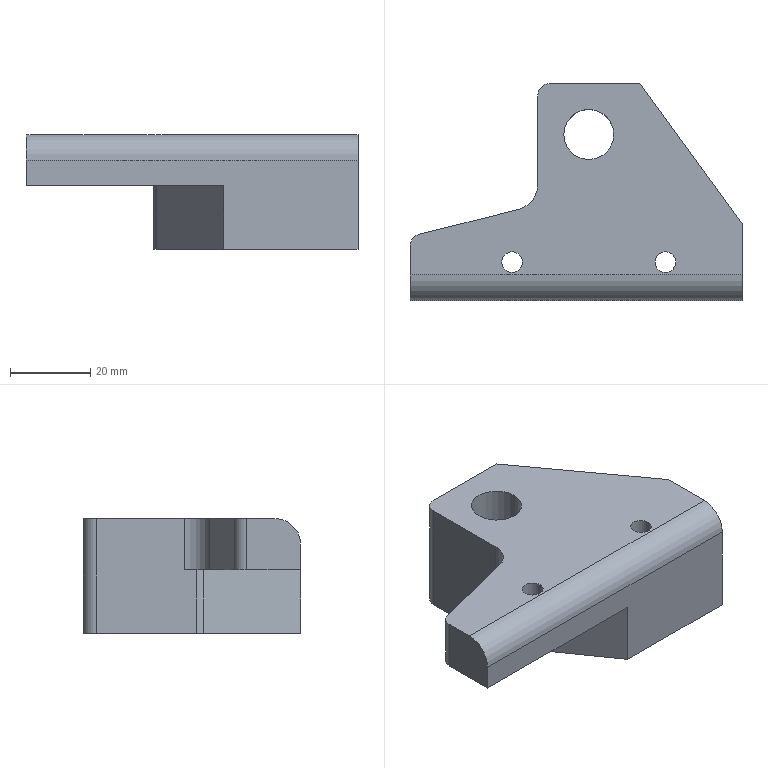NC program | NX | posted by the shop | part box 82.55 x 53.975 x 28.575 mm
Whole program:
%
O1234(11)
(T=1 D80 face mill Z=-30.00 D=80.00 R=0.00 L=30.00)
(T=2 D16-48-D16-100-3T-rough Z=-45.00 D=16.00 R=0.00 L=100.00)
(T=0 D12-36-D12-120-3T-finish Z=-55.00 D=12.00 R=0.00 L=120.00)
()
(T=4 drill D5.1-62-92 Z=-62.00 D=5.10 R=0.00 L=92.00)
(T=5 upper row M6-23-D6-63 Z=-23.00 D=6.00 R=0.00 L=26.00)
G40 G17 G80 G90 G21
M9
M5
G91 G28 Z0.0
M1
N1
(T=1 N=D80 face mill D=4.00 R=0.00 FL=12.00 L=50.00)
(XY-STOCK=0.10)
T1 M6
T2
G0 G90 G54 X88. Y0.0 S3500 M3
G43 H01 Z30.
M8
Z2.05
G1 Z.05 F800.
X43.
X-43.
X-88.
Z2.05
G0 Z30.
M9
M5
G91 G28 Z0.0
M1
N2
(T=2 N=D16-48-D16-100-3T-rough D=16.00 R=0.00 FL=45.00 L=100.00)
(XY-STOCK=0.60)
T2 M6
T6
G0 G90 G54 X-58.075 Y-25.19 S6500 M3
G43 H02 Z30.
M8
Z-24.9
G1 X-57.925 Y-25.183 Z-25.837 F2500.
X-57.775 Y-25.177 Z-26.208
X-57.625 Y-25.171 Z-26.48
X-57.475 Y-25.164 Z-26.7
X-57.325 Y-25.158 Z-26.884
X-57.176 Y-25.152 Z-27.042
X-57.026 Y-25.145 Z-27.18
X-56.876 Y-25.139 Z-27.3
X-56.726 Y-25.133 Z-27.405
X-56.576 Y-25.126 Z-27.498
X-56.426 Y-25.12 Z-27.579
X-56.276 Y-25.114 Z-27.65
X-56.127 Y-25.107 Z-27.71
X-55.977 Y-25.101 Z-27.762
X-55.827 Y-25.095 Z-27.805
X-55.677 Y-25.088 Z-27.839
X-55.527 Y-25.082 Z-27.866
X-55.377 Y-25.075 Z-27.885
X-55.227 Y-25.069 Z-27.896
X-55.077 Y-25.063 Z-27.9
X-52.483 Y-24.953
G3 X-51.072 Y-23.99 I-.069 J1.615
X-50.404 Y-20.967 I-10.219 J3.845
X-50.046 Y-12.897 I-86.855 J7.896
X-50.001 Y.166 I-855.802 J9.449
G1 X-50. Y24.239
G2 X-47.644 Y29.928 I8.521 J-.196
X-42.106 Y33.388 I9.531 J-9.091
X-35.342 Y34.661 I8.548 J-26.822
X-24.774 Y34.98 I9.67 J-144.964
G1 X-12.324 Y34.999
X39.312 Y34.998
G2 X45.036 Y32.543 I-.288 J-8.572
X48.435 Y26.964 I-9.338 J-9.516
X49.667 Y20.268 I-27.352 J-8.49
X49.98 Y9.775 I-146.761 J-9.633
G1 X49.999 Y-2.675
Y-24.311
G2 X47.693 Y-29.819 I-8.545 J.341
X42.228 Y-33.307 I-9.563 J8.957
X35.398 Y-34.634 I-8.657 J26.32
X24.906 Y-34.969 I-9.702 J139.455
G1 X13.281 Y-34.991
X-39.31 Y-34.998
G2 X-45.115 Y-32.463 I.288 J8.575
X-48.122 Y-27.095 I8.458 J8.265
X-48.966 Y-20.791 I26.665 J6.777
X-49.036 Y-15.842 I208.189 J5.408
G1 X-49.029 Y-1.961
X-49.001 Y12.389
G2 X-48.98 Y21.089 I508.473 J3.12
X-44.643 Y29.357 I11.471 J-.745
X-38.004 Y32.599 I10.799 J-13.696
X-30.148 Y33.728 I9.615 J-39.003
X-18.527 Y33.985 I10.654 J-219.016
G1 X-8.627 Y33.998
X35.561 Y33.997
G2 X44.259 Y29.758 I-.196 J-11.445
X47.559 Y23.15 I-13.41 J-10.825
X48.718 Y15.299 I-38.124 J-9.64
X48.986 Y3.079 I-220.307 J-10.953
G1 X48.998 Y-6.821
X48.997 Y-20.486
G2 X44.738 Y-29.238 I-11.49 J.179
X38.283 Y-32.496 I-10.792 J13.362
X30.439 Y-33.693 I-9.694 J37.205
X18.069 Y-33.977 I-11.078 J212.939
G1 X8.169 Y-33.991
X-35.56 Y-33.996
G2 X-41.664 Y-31.998 I.107 J10.65
G1 X-42.905 Y-31.48
X-44.056 Y-30.775
X-45.082 Y-29.898
X-45.958 Y-28.872
X-46.663 Y-27.721
X-47.179 Y-26.475
X-47.494 Y-25.162
G2 X-48.002 Y-13.629 I123.099 J11.2
X-48.015 Y1.606 I886.179 J8.341
G1 X-48.003 Y10.291
G2 X-47.968 Y18.213 I275.037 J2.746
X-42.166 Y28.601 I13.288 J-.608
X-35.036 Y31.664 I11.476 J-16.881
X-26.49 Y32.748 I10.35 J-47.361
X-13.293 Y32.989 I11.744 J-282.263
G1 X-3.393 Y32.998
X32.187 Y32.996
G2 X39.553 Y31.028 I.297 J-13.662
X45.054 Y24.68 I-8.113 J-12.588
X47.217 Y17.129 I-23.886 J-10.925
X47.897 Y7.408 I-79.997 J-10.482
X47.998 Y-10.216 I-882.58 J-13.849
X47.973 Y-18.011 I-320.284 J-2.881
X42.252 Y-28.509 I-13.315 J.449
X35.139 Y-31.617 I-11.522 J16.674
X26.898 Y-32.712 I-10.26 J45.669
X13.252 Y-32.98 I-12.047 J265.182
G1 X3.352 Y-32.991
X-32.11 Y-32.995
G2 X-36.486 Y-32.425 I.25 J18.99
G1 X-39.001 Y-32.418
X-40.346 Y-32.312
X-41.728 Y-31.968
X-40.346 Y-32.312
X-39.001 Y-32.418
X-9.236 Y-32.412
X-.282 Y-32.393
X11.018 Y-32.384
G3 X25.265 Y-32.164 I1.972 J333.178
X33.82 Y-31.154 I-1.655 J50.776
X40.547 Y-28.463 I-4.066 J19.915
X46.408 Y-20.132 I-7.435 J11.459
X47.244 Y-13.748 I-31.058 J7.311
X47.381 Y-.7 I-293.526 J9.624
X47.074 Y12.045 I-211.797 J1.262
X45.853 Y20.115 I-41.094 J-2.089
X42.614 Y26.753 I-17.515 J-4.436
X35.102 Y31.424 I-10.596 J-8.665
X28.566 Y32.254 I-7.373 J-31.919
X15.968 Y32.396 I-9.987 J-326.105
G1 X-4.782 Y32.397
G3 X-23.156 Y32.26 I-4.001 J-693.495
X-32.265 Y31.482 I1.116 J-66.776
X-39.38 Y29.184 I3.511 J-23.037
X-46.4 Y20.216 I6.301 J-12.164
X-47.242 Y13.908 I30.586 J-7.292
X-47.414 Y4.68 I270.329 J-9.64
G1 X-47.494 Y4.315
X-47.6 Y2.969
Y-23.818
Y2.969
X-47.494 Y4.315
G3 X-46.534 Y10.33 I-28.292 J7.601
G2 X-45.911 Y16.496 I71.44 J-4.099
X-43.095 Y23.454 I15.501 J-2.224
X-36.299 Y28.647 I13.065 J-10.055
X-28.406 Y30.675 I11.282 J-27.53
X-18.531 Y31.301 I10.784 J-92.036
X-.456 Y31.397 I13.905 J-915.227
G1 X15.419 Y31.396
G2 X27.492 Y31.242 I2.45 J-280.889
X33.574 Y30.416 I-.845 J-29.044
X42.537 Y23.47 I-3.881 J-14.264
X45.241 Y16.027 I-20.518 J-11.665
X46.184 Y7.161 I-57.778 J-10.629
X46.253 Y-12.185 I-283.58 J-10.69
X45.467 Y-18.349 I-30.54 J.761
X38.488 Y-27.503 I-14.32 J3.681
X30.896 Y-30.25 I-11.757 J20.63
X21.652 Y-31.194 I-10.807 J60.04
X6.054 Y-31.387 I-13.217 J439.445
G1 X-5.768 Y-31.414
X-6.133 Y-31.496
X-7.344 Y-31.998
X-8.656 Y-32.312
X-10.001 Y-32.418
X-8.656 Y-32.312
X-7.344 Y-31.998
G2 X-5.722 Y-31.351 I7.175 J-15.631
X-1.746 Y-30.922 I4.373 J-21.897
X10.769 Y-30.774 I10.856 J-387.99
G3 X23.588 Y-30.46 I.913 J224.643
X32.036 Y-29.229 I-2.227 J44.889
X39.059 Y-25.944 I-4.647 J19.083
X44.364 Y-18.103 I-9.482 J12.131
X45.548 Y-10.941 I-29.925 J8.626
X45.724 Y1.28 I-168.542 J8.545
X45.168 Y11.986 I-107.119 J-.202
X43.408 Y19.641 I-31.158 J-3.131
X38.702 Y26.418 I-15.302 J-5.605
X31.638 Y29.77 I-10.601 J-13.217
X24.126 Y30.651 I-8.457 J-39.649
X10.852 Y30.795 I-10.659 J-369.787
G1 X-.973 Y30.796
G3 X-19.722 Y30.653 I-4.021 J-701.215
X-29.206 Y29.854 I1.226 J-71.196
X-36.617 Y27.525 I3.719 J-24.796
X-44.305 Y18.484 I6.972 J-13.718
X-45.625 Y12.257 I30.739 J-9.769
G2 X-46.277 Y7.6 I-70.503 J7.497
X-46.662 Y6.874 I-3.081 J1.168
G1 X-47.179 Y5.627
X-46.662 Y6.874
G3 X-45.378 Y9.898 I-7.382 J4.92
G2 X-44.132 Y15.049 I323.49 J-75.484
X-40.97 Y21.631 I17.893 J-4.546
X-33.549 Y27.073 I13.907 J-11.184
X-25.483 Y29.063 I11.649 J-29.876
X-14.633 Y29.71 I11.508 J-101.634
X1.642 Y29.795 I12.722 J-878.987
G1 X13.867 Y29.79
G2 X24.738 Y29.551 I1.5 J-179.669
X31.674 Y28.388 I-1.417 J-29.71
X41.122 Y20.485 I-4.789 J-15.324
X43.716 Y12.678 I-23.168 J-12.033
X44.611 Y3.053 I-66.913 J-11.078
X44.513 Y-10.066 I-135.835 J-5.55
X43.272 Y-16.99 I-27.926 J1.435
X35.554 Y-26.062 I-15.2 J5.111
X27.831 Y-28.672 I-12.032 J22.874
X18.434 Y-29.592 I-11.123 J65.168
X4.343 Y-29.807 I-14.621 J496.937
G3 X-3.02 Y-30.111 I-.434 J-78.905
X-4.413 Y-30.392 I.239 J-4.775
X-4.946 Y-30.776 I1.419 J-2.527
G1 X-6.097 Y-31.481
X-4.946 Y-30.776
G2 X-3.579 Y-30.029 I1.967 J-1.974
X.811 Y-29.405 I5.222 J-20.963
X10.981 Y-29.154 I10.602 J-224.095
G3 X22.594 Y-28.693 I-.288 J153.526
X30.978 Y-27.112 I-2.844 J38.107
X38.201 Y-22.942 I-5.476 J17.829
X42.76 Y-15.102 I-12.129 J12.297
X43.917 Y-7.555 I-33.865 J9.053
X43.582 Y8.776 I-109.231 J5.932
X41.811 Y16.889 I-33.856 J-3.141
X36.94 Y24.18 I-16.627 J-5.836
X29.545 Y27.926 I-11.631 J-13.786
X21.98 Y28.978 I-9.087 J-37.628
X9.534 Y29.192 I-10.491 J-248.473
G1 X-4.041 Y29.189
G3 X-19.113 Y28.947 I-2.022 J-342.855
X-28.339 Y27.861 I1.922 J-56.087
X-35.848 Y24.899 I4.553 J-22.541
X-42.4 Y17.032 I9.385 J-14.479
X-44.286 Y11.46 I42.591 J-17.517
G2 X-45.105 Y9.071 I-20.585 J5.725
X-45.957 Y8.024 I-7.808 J5.482
G1 X-46.192 Y7.641
X-45.957 Y8.024
G3 X-44.671 Y9.587 I-12.905 J11.927
X-43.156 Y12.716 I-18.651 J10.964
G2 X-40.515 Y17.994 I30.917 J-12.168
X-31.669 Y25.25 I15.974 J-10.453
X-23.187 Y27.404 I12.311 J-30.712
X-12.864 Y28.081 I11.55 J-97.008
X8.285 Y28.191 I15.646 J-975.269
X20.582 Y27.992 I1.967 J-257.933
X28.15 Y26.962 I-1.374 J-38.435
X36.925 Y21.772 I-4.024 J-16.816
X41.129 Y14.049 I-15.623 J-13.51
X42.701 Y5.205 I-39.731 J-11.624
X42.715 Y-8.579 I-82.104 J-6.979
X41.064 Y-15.795 I-25.506 J2.041
X32.929 Y-24.532 I-15.759 J6.518
X24.803 Y-27.122 I-12.458 J25.045
X14.95 Y-28.012 I-11.581 J73.195
G1 X4.577 Y-28.271
G3 X-1.596 Y-28.808 I.641 J-43.085
X-3.304 Y-29.307 I.788 J-5.866
X-3.92 Y-29.9 I1.419 J-2.089
G1 X-4.604 Y-30.485
G3 X-3.453 Y-29.366 I-3.975 J5.245
G2 X-1.418 Y-28.505 I3.218 J-4.768
X4.213 Y-27.776 I6.745 J-29.997
X14.692 Y-27.407 I29.26 J-682.149
G3 X24.243 Y-26.509 I-1.977 J72.26
X32.136 Y-23.961 I-4.255 J26.684
X40.652 Y-13.963 I-8.013 J15.45
X42.153 Y-5.951 I-29.731 J9.717
X41.589 Y8.785 I-68.202 J4.766
X39.157 Y16.792 I-27.506 J-3.98
X28.865 Y25.715 I-15.71 J-7.723
X21.303 Y27.2 I-9.932 J-30.572
X11.188 Y27.569 I-9.723 J-127.797
X-12.511 Y27.476 I-8.098 J-954.556
X-23.203 Y26.715 I1.09 J-90.808
X-31.494 Y24.423 I3.952 J-30.432
X-40.378 Y16.412 I8.106 J-17.923
X-42.844 Y11.78 I64.623 J-37.376
G2 X-43.549 Y10.582 I-7.123 J3.385
G1 X-45.034 Y9.097
G3 X-42.66 Y11.506 I-41.495 J43.25
X-40.224 Y14.921 I-44.884 J34.598
G2 X-34.697 Y20.808 I20.623 J-13.825
X-25.848 Y24.843 I14.688 J-20.487
X-16.285 Y26.22 I12.294 J-51.5
X-2.042 Y26.575 I13.152 J-241.989
X15.582 Y26.469 I5.422 J-567.569
X24.011 Y25.677 I-.951 J-55.335
X31.542 Y22.829 I-3.556 J-20.783
X38.229 Y14.981 I-10.048 J-15.336
X40.64 Y6.344 I-27.985 J-12.468
X40.798 Y-7.716 I-53.58 J-7.63
X38.513 Y-15.292 I-22.492 J2.65
X30.344 Y-23.037 I-15.843 J8.532
X22.04 Y-25.549 I-12.728 J27.084
X12.41 Y-26.426 I-12.215 J80.859
G3 X3.514 Y-26.885 I6.472 J-211.864
X-1.292 Y-27.721 I1.608 J-23.471
X-2.595 Y-28.312 I1.014 J-3.972
G1 X-2.9 Y-28.641
G3 X-2.988 Y-30.142 I1.367 J-.832
G1 X-2.826 Y-30.417 Z-27.89
X-2.637 Y-30.674 Z-27.88
X-1.144 Y-32.711 Z-27.8
X-.441 Y-33.669 F10000.
G3 X2.135 Y-33.676 I1.29 J.946
G1 X2.431 Y-33.281
X2.714 Y-32.876
G3 X.478 Y-30.724 I-1.39 J.794
G1 X-1.608 Y-31.935 Z-27.876 F2500.
G2 X-2.331 Y-32.114 Z-27.9 I-.738 J1.429
X-3.556 Y-29.475 I-.009 J1.6
G3 X-2.764 Y-28.43 I-3.695 J3.626
G2 X-1.281 Y-27.502 I2.773 J-2.783
X3.421 Y-26.44 I6.477 J-17.747
X12.017 Y-25.848 I13.593 J-134.594
G3 X21.419 Y-24.955 I-3.197 J83.605
X29.575 Y-22.469 I-4.358 J28.916
X38.959 Y-11.63 I-7.916 J16.335
X40.404 Y-3.004 I-29.963 J9.455
X39.329 Y9.361 I-45.671 J2.256
X35.867 Y17.296 I-22.364 J-5.033
X26.838 Y23.958 I-14.852 J-10.68
X18.919 Y25.561 I-10.471 J-31.367
X7.98 Y25.966 I-10.333 J-131.044
X-12.118 Y25.802 I-5.651 J-537.
X-22.416 Y24.85 I1.777 J-75.442
X-31.087 Y22.04 I4.738 J-29.398
X-38.491 Y15.859 I11.302 J-21.063
G1 X-39.399 Y14.732
X-42.952 Y11.178
X-35.231 Y18.9
X-34.204 Y19.776
X-33.053 Y20.481
G2 X-16.847 Y24.403 I20.485 J-49.206
X-3.737 Y24.94 I13.303 J-164.533
X13.661 Y24.83 I6.167 J-400.766
X22.154 Y23.933 I-1.287 J-52.868
X30.047 Y20.735 I-3.962 J-21.115
X36.75 Y12.382 I-10.995 J-15.689
X39.034 Y3.019 I-29.061 J-12.048
X38.623 Y-7.734 I-36.466 J-3.992
X34.703 Y-16.317 I-19.167 J3.568
X26.759 Y-22.011 I-15.139 J12.733
X18.125 Y-24.175 I-12.877 J33.072
X8.654 Y-25.008 I-17.512 J144.793
G3 X1.634 Y-25.863 I2.683 J-51.288
X-1.806 Y-27.11 I1.969 J-10.801
X-2.308 Y-27.659 I1.242 J-1.641
X-2.21 Y-29.216 I1.444 J-.691
G1 X-1.25 Y-30.474 Z-27.85
X-.279 Y-31.724 Z-27.8
X.342 Y-32.528 F10000.
G3 X2.727 Y-32.694 I1.266 J.979
G1 X3.094 Y-32.339
X3.448 Y-31.972
G3 X1.407 Y-29.581 I-1.248 J1.002
G1 X1.052 Y-29.784
X.141 Y-30.309 Z-27.833 F2500.
X-.776 Y-30.822 Z-27.866
G2 X-1.809 Y-30.957 Z-27.9 I-.712 J1.433
X-2.847 Y-28.554 I.326 J1.566
G3 X-2.209 Y-27.453 I-8.362 J5.581
G2 X-.83 Y-26.395 I2.899 J-2.352
X3.484 Y-25.098 I6.681 J-14.401
X10.306 Y-24.323 I12.049 J-75.567
G3 X19.32 Y-23.309 I-6.438 J97.876
X27.404 Y-20.822 I-4.782 J29.913
X37.303 Y-9.12 I-8.025 J16.827
X38.426 Y.897 I-29.301 J8.356
X36.476 Y10.863 I-31.29 J-.948
X29.828 Y19.649 I-17.931 J-6.66
X21.744 Y23.132 I-12.652 J-18.243
X12.893 Y24.188 I-10.419 J-49.7
X-3.904 Y24.331 I-11.161 J-326.041
X-16.937 Y23.743 I.334 J-152.148
X-28.391 Y21.447 I5.234 J-55.845
G2 X-29.15 Y21.418 I-.622 J6.36
G1 X-30.494 Y21.312
X-31.807 Y20.998
X-30.494 Y21.312
G2 X-27.415 Y21.418 I2.334 J-23.06
G3 X-22.295 Y22.035 I-5.495 J67.178
G2 X-5.552 Y23.273 I18.319 J-133.888
X12.07 Y23.176 I7.223 J-288.332
X20.475 Y22.171 I-1.661 J-49.549
X28.561 Y18.67 I-4.377 J-21.194
X35.217 Y9.865 I-11.749 J-15.799
X36.507 Y-6.725 I-27.213 J-10.462
X26.812 Y-19.345 I-18.19 J3.941
X18.448 Y-22.16 I-13.687 J26.841
X10.798 Y-23.216 I-15.834 J86.473
G3 X3.406 Y-24.232 I6.216 J-72.596
X-.699 Y-25.633 I2.746 J-14.76
X-1.825 Y-26.544 I1.274 J-2.724
X-2.324 Y-27.691 I13.446 J-6.54
G1 X-1.8 Y-26.447
G2 X-.074 Y-25.06 I3.708 J-2.848
X4.501 Y-23.574 I7.65 J-15.758
X11.796 Y-22.519 I17.601 J-95.986
G3 X20.21 Y-21.039 I-6.585 J62.09
X28.083 Y-17.552 I-5.966 J24.1
X35.566 Y-6.543 I-10.705 J15.324
X34.169 Y10.131 I-25.668 J6.245
X23.189 Y20.41 I-17.505 J-7.693
X15.162 Y22.219 I-11.18 J-30.895
X4.379 Y22.725 I-10.44 J-107.413
X-13.612 Y22.309 I-3.392 J-242.692
X-22.214 Y21.418 I10.615 J-144.454
G1 X-27.464
X-18.756
G3 X-13.982 Y21.397 I2.575 J41.747
G2 X6.758 Y21.662 I15.105 J-370.514
X16.396 Y20.905 I-.699 J-70.701
X24.364 Y18.363 I-3.751 J-25.508
X33.36 Y7.981 I-9.084 J-16.961
X34.119 Y-6.243 I-21.787 J-8.295
X25.585 Y-17.223 I-17.616 J4.887
X17.552 Y-20.32 I-14.287 J25.087
X9.246 Y-21.79 I-21.755 J98.712
G3 X2.746 Y-23.143 I6.002 J-45.146
X-.799 Y-24.808 I3.241 J-11.503
X-1.689 Y-25.925 I1.141 J-1.821
G2 X-1.879 Y-26.615 I-6.348 J1.376
G3 X-1.611 Y-25.636 I-11.147 J3.574
G2 X-.419 Y-24.321 I3.13 J-1.639
X3.389 Y-22.546 I7.299 J-10.688
X9.411 Y-21.218 I13.543 J-47.095
G3 X17.281 Y-19.685 I-15.445 J100.257
X25.119 Y-16.501 I-6.399 J26.992
X33.759 Y-3.057 I-9.593 J15.663
X30.762 Y11.119 I-21.138 J2.937
X21.567 Y18.587 I-16.067 J-10.387
X13.347 Y20.549 I-11.531 J-30.108
X2.491 Y21.091 I-10.407 J-99.548
X-13.678 Y20.812 I-.442 J-443.152
G2 X-15.598 Y20.822 I-.888 J13.396
G3 X-17.41 Y21.312 I-4.662 J-13.651
G1 X-18.232 Y21.377
X-17.41 Y21.312
X-16.098 Y20.997
G3 X-13.33 Y20.305 I3.321 J7.41
X-6.37 Y20.074 I5.74 J67.971
G2 X6.732 Y19.966 I3.924 J-318.37
X15.819 Y18.981 I-1.41 J-55.422
X24.003 Y15.723 I-4.419 J-23.006
X32.232 Y2.271 I-10.471 J-15.649
X29.566 Y-9.861 I-17.759 J-2.455
X22.288 Y-16.269 I-15.889 J10.707
X14.52 Y-19.044 I-15.207 J30.317
X7.059 Y-20.653 I-109.199 J488.165
G3 X1.451 Y-22.459 I5.504 J-26.704
X-1.157 Y-24.289 I3.293 J-7.469
X-1.491 Y-25.034 I1.529 J-1.134
X-1.151 Y-26.28 I1.584 J-.237
G1 X-.704 Y-26.831
X1.291 Y-29.288 Z-27.8
X1.579 Y-29.637 F10000.
X1.853 Y-29.997
G2 X2.069 Y-31.201 I-1.349 J-.863
G1 X1.969 Y-31.669
X1.854 Y-32.133
G2 X-.956 Y-32.539 I-1.511 J.528
X-1.264 Y-31.582 Z-27.832 I1.425 J.987 F2500.
G1 X-1.437 Y-29.445 Z-27.9
X-1.693 Y-26.282
G2 X-1.654 Y-25.779 I1.703 J.121
G3 X-1.446 Y-24.72 I-8.677 J2.251
G2 X-.345 Y-23.301 I3.279 J-1.409
X3.463 Y-21.235 I7.855 J-9.931
X9.367 Y-19.604 I15.726 J-45.432
G3 X16.791 Y-17.717 I-17.729 J85.275
X24.308 Y-14.002 I-7.371 J24.378
X31.08 Y3.094 I-10.29 J13.966
X21.206 Y16.175 I-17.719 J-3.107
X12.912 Y18.685 I-12.18 J-25.284
X2.897 Y19.427 I-10.554 J-74.535
X-8.078 Y19.496 I-11.705 J-993.286
G2 X-13.635 Y19.881 I-.205 J37.268
X-14.173 Y20.065 I.668 J2.838
G3 X-15.405 Y20.71 I-2.827 J-3.899
G2 X-14.173 Y20.065 I-1.594 J-4.544
G3 X-11.98 Y19.224 I3.27 J5.25
X-6.294 Y18.63 I6.35 J33.249
X3.284 Y18.398 I27.531 J939.58
G2 X12.54 Y17.577 I-1.287 J-67.124
X20.486 Y14.952 I-4.037 J-25.561
X29.324 Y3.105 I-7.995 J-15.184
X24.141 Y-11.893 I-15.678 J-2.976
X16.843 Y-16.213 I-15.479 J17.82
X9.815 Y-18.38 I-22.789 J61.431
G3 X3.417 Y-20.361 I12.556 J-51.881
X-.432 Y-22.621 I4.512 J-12.091
X-1.341 Y-23.795 I2.061 J-2.533
X-1.497 Y-25.053 I5.331 J-1.303
G1 X-1.395 Y-23.858
G2 X-.274 Y-22.216 I3.573 J-1.236
X3.448 Y-19.926 I8.537 J-9.705
X8.867 Y-18.078 I17.82 J-43.396
G3 X15.743 Y-15.888 I-22.192 J81.548
X22.757 Y-11.88 I-8.299 J22.667
X28.443 Y-.387 I-9.973 J12.088
X22.098 Y12.638 I-15.831 J.346
X14.131 Y16.369 I-13.134 J-17.676
X5.234 Y17.638 I-11.086 J-45.896
X-4.839 Y17.992 I-18.984 J-397.019
G2 X-11.116 Y18.587 I.726 J41.07
X-12.889 Y19.115 I1.137 J7.06
X-13.701 Y19.775 I6.67 J9.027
G1 X-13.828 Y19.853
G2 X-12.79 Y18.997 I-6.992 J-9.539
G3 X-10.241 Y17.926 I4.124 J6.243
X-4.513 Y17.137 I7.294 J31.77
G1 X4.005 Y16.68
G2 X12.539 Y15.51 I-2.47 J-49.72
X20.066 Y12.223 I-4.78 J-21.21
X26.216 Y3.026 I-8.507 J-12.343
X23.155 Y-8.775 I-13.863 J-2.702
X16.809 Y-13.773 I-15.374 J12.994
X9.788 Y-16.623 I-21.872 J43.799
G3 X3.696 Y-18.888 I19.598 J-62.045
X-.238 Y-21.374 I5.617 J-13.244
X-1.302 Y-22.771 I2.753 J-3.202
X-1.4 Y-23.819 I2.599 J-.772
G1 X-1.418 Y-24.043
X-1.391 Y-22.955
G2 X-.383 Y-21.234 I3.663 J-.991
X3.203 Y-18.686 I9.1 J-9.008
X8.134 Y-16.625 I20.019 J-40.955
G3 X14.66 Y-14.032 I-25.112 J72.697
X20.992 Y-9.716 I-9.075 J20.121
X25.176 Y-.481 I-9.804 J10.007
X20.73 Y10.111 I-13.772 J.449
X13.391 Y14.309 I-12.974 J-14.171
X5.083 Y15.894 I-11.397 J-37.178
X-3.472 Y16.481 I-27.629 J-339.94
G2 X-9.575 Y17.3 I1.986 J37.957
X-11.864 Y18.125 I1.735 J8.4
X-12.846 Y19.045 I21.1 J23.49
G1 X-11.722 Y17.946
G3 X-8.919 Y16.615 I4.75 J6.384
X-3.286 Y15.629 I8.276 J30.704
G2 X4.713 Y14.881 I-68.819 J-778.925
X12.48 Y13.257 I-3.589 J-36.555
X19.149 Y9.289 I-5.415 J-16.687
X21.218 Y-5.869 I-8.499 J-8.881
X15.841 Y-11.485 I-14.907 J8.892
X9.38 Y-14.883 I-21.099 J32.277
G3 X3.525 Y-17.546 I31.08 J-76.09
X-.347 Y-20.329 I6.644 J-13.331
X-1.318 Y-21.736 I3.134 J-3.199
G1 X-1.4 Y-22.177
Y-23.152
X-1.392 Y-21.877
G2 X-.254 Y-19.91 I4.291 J-1.169
X3.448 Y-17.121 I10.603 J-10.222
X9.287 Y-14.284 I40.705 J-76.344
G3 X15.302 Y-10.891 I-14.468 J32.674
X20.163 Y-5.432 I-9.096 J12.994
X18.785 Y7.467 I-10.457 J5.406
X12.471 Y12.102 I-12.387 J-10.255
X5.246 Y14.046 I-11.357 J-27.821
X-2.733 Y14.979 I-26.925 J-195.567
G2 X-8.526 Y16.035 I3.331 J34.681
X-10.692 Y16.934 I2.104 J8.128
G1 X-11.761 Y17.985
G3 X-10.271 Y16.525 I24.583 J23.593
X-7.015 Y15.048 I5.722 J8.289
X-1.019 Y13.904 I11.198 J42.412
G2 X6.298 Y12.732 I-11.153 J-93.034
X12.824 Y10.336 I-4.517 J-22.391
X17.804 Y5.263 I-5.986 J-10.857
X18.001 Y-3.963 I-9.856 J-4.825
X13.487 Y-9.857 I-14.356 J6.32
X8.016 Y-13.474 I-21.607 J26.734
G3 X2.7 Y-16.533 I38.827 J-73.638
X-.698 Y-19.503 I7.326 J-11.809
X-1.376 Y-20.771 I2.368 J-2.081
X-1.4 Y-22.035 I13.264 J-.883
G1 X-1.398 Y-20.76
G2 X-.516 Y-18.946 I4.005 J-.826
X2.95 Y-15.877 I11.383 J-9.365
X8.348 Y-12.59 I75.199 J-117.439
G3 X13.553 Y-8.659 I-13.606 J23.422
X16.972 Y-2.996 I-8.912 J9.244
X14.982 Y6.271 I-10.293 J2.637
X9.104 Y10.71 I-11.675 J-9.349
X2.345 Y12.67 I-11.878 J-28.326
G2 X-4.29 Y13.857 I65.453 J384.908
X-8.765 Y15.24 I3.709 J19.945
X-9.391 Y15.615 I1.434 J3.097
G1 X-10.452 Y16.676
X-8.871 Y15.118
G3 X-5.572 Y13.53 I6.215 J8.691
X-.927 Y12.361 I14.353 J47.217
G2 X5.263 Y10.825 I-11.116 J-58.019
X10.707 Y8.01 I-4.964 J-16.276
X14.142 Y-2.069 I-6.125 J-7.712
X10.824 Y-8.221 I-13.64 J3.386
X5.944 Y-12.468 I-22.212 J20.59
G3 X1.437 Y-15.881 I39.96 J-57.455
X-1.199 Y-18.936 I7.267 J-8.937
X-1.4 Y-19.653 I1.774 J-.883
G1 Y-20.853
X-1.398 Y-19.428
G2 X-.422 Y-17.399 I4.73 J-1.028
X2.914 Y-14.122 I14.801 J-11.731
G3 X7.514 Y-10.42 I-82.385 J107.085
X11.47 Y-5.713 I-11.563 J13.732
X11.087 Y4.544 I-8.529 J4.818
X5.768 Y9.21 I-11.45 J-7.688
X-.057 Y11.378 I-13.288 J-26.792
G2 X-5.415 Y12.94 I20.792 J81.308
X-7.764 Y14.004 I3.436 J10.713
G1 X-9.025 Y15.249
G3 X-7.276 Y13.524 I168.907 J169.502
X-4.017 Y11.814 I7.417 J10.176
G2 X1.353 Y9.883 I-328.526 J-921.732
X6.311 Y7.108 I-6.072 J-16.666
X9.646 Y-1.121 I-6.035 J-7.236
X7.199 Y-7.572 I-13.6 J1.469
X3.245 Y-12.141 I-25.991 J18.497
G3 X-.165 Y-15.806 I27.828 J-29.306
X-1.341 Y-17.759 I5.533 J-4.664
G1 X-1.4 Y-18.129
Y-19.554
X-1.399 Y-17.904
G2 X-.51 Y-15.839 I5.315 J-1.064
X2.288 Y-12.404 I22.316 J-15.321
G3 X5.918 Y-8.025 I-27.656 J26.619
X7.989 Y-3.243 I-10.228 J7.27
X6.067 Y4.403 I-9.967 J1.56
X1.157 Y8.624 I-12.272 J-9.308
X-3.814 Y11.032 I-29.839 J-55.257
G2 X-5.93 Y12.158 I5.387 J12.681
G1 X-7.454 Y13.678
G3 X-5.097 Y11.362 I36.199 J34.489
X-1.763 Y9.209 I18.396 J24.828
G2 X2.345 Y6.192 I-10.415 J-18.486
X5.274 Y-1.787 I-7.112 J-7.138
X3.343 Y-8.059 I-15.401 J1.308
X.498 Y-12.559 I-45.302 J25.493
G3 X-1.332 Y-15.778 I14.342 J-10.282
G1 X-1.4 Y-16.158
Y-18.033
X-1.399 Y-15.933
G2 X-.454 Y-13.433 I7.933 J-1.571
X1.92 Y-9.278 I612.857 J-347.288
G3 X3.867 Y-4.023 I-14.6 J8.4
X2.1 Y3.771 I-10.866 J1.633
X-1.938 Y8.078 I-15.731 J-10.699
G2 X-2.956 Y8.978 I3.595 J5.093
G3 X-3.918 Y10.142 I-11.117 J-8.208
G1 X-5.403 Y11.627
G2 X-3.042 Y9.116 I-18.914 J-20.15
G3 X-1.355 Y6.715 I17.507 J10.513
G2 X1.084 Y2.514 I-12.15 J-9.858
X1.46 Y-5.027 I-12.949 J-4.426
X-.21 Y-10.076 I-28.071 J6.485
G3 X-1.366 Y-13.038 I33.017 J-14.591
G1 X-1.4 Y-13.285
Y-16.06
Y-13.06
G2 X-.708 Y-10.221 I14.069 J-1.924
G3 X.627 Y-5.122 I-31.867 J11.071
X-.721 Y3.562 I-14.427 J2.207
G2 X-1.438 Y5.052 I29.306 J15.03
G1 X-1.492 Y5.27
G2 X-1.153 Y6.459 I1.591 J.19
G1 X-.681 Y7.05
X1.294 Y9.522 Z-27.8
X1.646 Y9.968 F10000.
X2.012 Y10.403
G2 X4.675 Y8.83 I1.122 J-1.14
G1 X4.584 Y8.502
X4.48 Y8.177
G2 X2.07 Y7.49 I-1.478 J.613
X1.609 Y7.989 Z-27.822 I1.148 J1.525 F2500.
G1 X.17 Y10.01 Z-27.9
G3 X-1.014 Y10.782 I-1.416 J-.878
X-2.578 Y8.359 I-.199 J-1.588
G1 X-2.337 Y7.965
X-1.821 Y6.718
X-1.506 Y5.406
G3 X-1.104 Y2.932 I16.924 J1.483
G2 X-1.106 Y-6.452 I-22.8 J-4.685
G1 X-1.4 Y-8.025
Y-13.125
G2 X-1.377 Y-6.024 I303.737 J2.587
G3 X-1.4 Y-.655 I-41.002 J2.512
G1 Y4.061
X-1.465 Y4.884
X-1.4 Y4.061
Y-6.805
G3 X-.014 Y-8.404 I1.616 J0.0
G1 X2.556 Y-8.775
X2.704 Y-8.796 Z-27.896
X2.853 Y-8.817 Z-27.885
X3.001 Y-8.839 Z-27.866
X3.15 Y-8.86 Z-27.839
X3.298 Y-8.881 Z-27.805
X3.447 Y-8.903 Z-27.762
X3.595 Y-8.924 Z-27.71
X3.744 Y-8.946 Z-27.65
X3.892 Y-8.967 Z-27.579
X4.04 Y-8.988 Z-27.498
X4.189 Y-9.01 Z-27.405
X4.337 Y-9.031 Z-27.3
X4.486 Y-9.052 Z-27.18
X4.634 Y-9.074 Z-27.042
X4.783 Y-9.095 Z-26.884
X4.931 Y-9.117 Z-26.7
X5.08 Y-9.138 Z-26.48
X5.228 Y-9.159 Z-26.208
X5.377 Y-9.181 Z-25.837
X5.525 Y-9.202 Z-24.9
G0 Z30.
X-58.075 Y-25.184
Z-67.
G1 X-57.925 Y-25.178 Z-67.937
X-57.775 Y-25.171 Z-68.308
X-57.625 Y-25.165 Z-68.58
X-57.476 Y-25.159 Z-68.8
X-57.326 Y-25.153 Z-68.984
X-57.176 Y-25.147 Z-69.142
X-57.026 Y-25.14 Z-69.28
X-56.876 Y-25.134 Z-69.4
X-56.726 Y-25.128 Z-69.505
X-56.576 Y-25.122 Z-69.598
X-56.426 Y-25.115 Z-69.679
X-56.277 Y-25.109 Z-69.75
X-56.127 Y-25.103 Z-69.81
X-55.977 Y-25.097 Z-69.862
X-55.827 Y-25.091 Z-69.905
X-55.677 Y-25.084 Z-69.939
X-55.527 Y-25.078 Z-69.966
X-55.377 Y-25.072 Z-69.985
X-55.227 Y-25.066 Z-69.996
X-55.078 Y-25.06 Z-70.
X-52.485 Y-24.952
G3 X-51.072 Y-23.986 I-.067 J1.615
X-50.404 Y-20.965 I-10.261 J3.853
X-50.05 Y-13.19 I-84.345 J7.742
X-50.001 Y2.864 I-999.416 J11.074
G1 X-50. Y24.313
G2 X-47.645 Y29.927 I8.528 J-.276
X-42.106 Y33.388 I9.531 J-9.091
X-35.343 Y34.661 I8.549 J-26.825
X-25.45 Y34.976 I9.331 J-137.342
G1 X-11.8 Y34.999
X39.312
G2 X45.036 Y32.543 I-.288 J-8.57
X48.435 Y26.965 I-9.339 J-9.516
X49.667 Y20.268 I-27.353 J-8.49
X49.981 Y9.4 I-150.742 J-9.804
G1 X49.999 Y-3.35
Y-24.311
G2 X47.693 Y-29.819 I-8.546 J.341
X42.228 Y-33.307 I-9.563 J8.957
X35.398 Y-34.634 I-8.657 J26.321
X24.906 Y-34.969 I-9.703 J139.462
G1 X13.281 Y-34.991
X-39.31 Y-34.998
G2 X-44.98 Y-32.594 I.279 J8.545
X-48.042 Y-27.384 I8.126 J8.28
X-48.954 Y-21.091 I25.302 J6.878
X-49.036 Y-15.842 I161.742 J5.165
G1 X-49.028 Y1.038
X-49.001 Y14.939
G2 X-48.971 Y21.238 I176.563 J2.288
X-44.643 Y29.356 I11.468 J-.9
X-38.004 Y32.599 I10.8 J-13.695
X-30.148 Y33.728 I9.615 J-39.001
X-17.927 Y33.985 I10.96 J-230.775
G1 X-6.077 Y33.999
X35.561 Y33.997
G2 X44.26 Y29.758 I-.197 J-11.446
X47.559 Y23.149 I-13.412 J-10.824
X48.718 Y15.298 I-38.141 J-9.641
X48.983 Y3.152 I-221.699 J-10.922
G1 X48.998 Y-7.948
G2 X48.979 Y-21.01 I-947.119 J-5.147
X44.622 Y-29.334 I-11.507 J.721
X38.066 Y-32.556 I-10.789 J13.674
X30.214 Y-33.708 I-9.657 J38.482
X18.069 Y-33.978 I-10.964 J220.366
G1 X8.169 Y-33.991
X-35.56 Y-33.996
G2 X-41.661 Y-31.993 I.064 J10.485
G3 X-42.582 Y-31.636 I-7.591 J-18.246
G1 X-43.804 Y-30.951
X-44.898 Y-30.077
X-45.836 Y-29.037
X-46.592 Y-27.858
X-47.147 Y-26.572
X-47.486 Y-25.213
G2 X-48.002 Y-13.629 I121.329 J11.212
X-48.024 Y2.141 I962.677 J9.2
G1 X-48.003 Y10.516
G2 X-47.967 Y18.238 I256.312 J2.652
X-42.214 Y28.567 I13.283 J-.632
X-35.074 Y31.655 I11.502 J-16.797
X-26.529 Y32.743 I10.297 J-46.753
X-12.958 Y32.987 I12.088 J-295.193
G1 X-1.708 Y32.998
X32.111 Y32.997
G2 X39.167 Y31.26 I.335 J-13.835
X44.855 Y25.082 I-7.512 J-12.625
X47.136 Y17.647 I-22.528 J-10.98
X47.861 Y8.607 I-70.03 J-10.163
X47.996 Y-10.292 I-763.575 J-14.911
X47.973 Y-18.011 I-375.986 J-2.722
X42.252 Y-28.509 I-13.315 J.448
X35.139 Y-31.617 I-11.522 J16.674
X26.748 Y-32.721 I-10.325 J46.057
X13.102 Y-32.981 I-12.026 J272.445
G1 X3.202 Y-32.992
X-32.11 Y-32.996
G2 X-36.412 Y-32.434 I.045 J17.092
G1 X-39.009 Y-32.418
G2 X-41.266 Y-32.114 I.195 J9.978
G1 X-41.83 Y-31.91
G3 X-40.148 Y-32.341 I2.76 J7.261
X-36.561 Y-32.418 I2.57 J36.161
G1 X-9.537 Y-32.413
X2.093 Y-32.392
G3 X22.217 Y-32.276 I4.589 J945.148
X31.486 Y-31.59 I-.978 J76.216
X38.733 Y-29.488 I-3.323 J24.999
X45.002 Y-23.735 I-5.862 J12.679
X46.892 Y-17.684 I-15.463 J8.15
X47.35 Y-10.052 I-61.351 J7.512
G1 X47.385 Y-7.953
X47.483 Y-7.458
X47.6 Y-5.682
Y5.847
G3 X46.821 Y15.037 I-238.171 J-15.553
X45.13 Y22.326 I-30.098 J-3.145
X40.762 Y28.638 I-14.346 J-5.259
X34.432 Y31.584 I-9.116 J-11.316
X27.503 Y32.296 I-7.433 J-38.257
X21.543 Y32.385 I-9.605 J-445.36
G1 X21.029 Y32.418
X-21.028
G3 X-29.004 Y31.919 I8.603 J-201.506
X-36.703 Y30.359 I2.654 J-32.864
X-43.029 Y26.446 I5.033 J-15.207
X-46.492 Y19.852 I10.261 J-9.595
X-47.274 Y13.234 I33.939 J-7.365
X-47.397 Y8.057 I563.216 J-16.01
G1 X-47.483 Y7.623
X-47.6 Y5.848
Y-23.818
G2 X-50.711 Y-24.344 I-1.6 J0.0
G1 X-51.552 Y-21.293 Z-69.9
X-51.773 Y-20.501 F10000.
X-51.981 Y-19.706
X-52.006 Y-19.412
X-51.803 Y3.652
G2 X-51.571 Y4.466 I1.61 J-.017
X-50.981 Y5.045 Z-69.926 I1.516 J-.958 F2500.
G1 X-49.06 Y6.364 Z-70.
X-48.06 Y7.051
G3 X-47.397 Y8.057 I-.908 J1.32
X-46.739 Y11.341 I-101.902 J22.141
G2 X-45.948 Y16.733 I140.089 J-17.777
X-42.994 Y23.631 I15.623 J-2.609
X-36.134 Y28.727 I13.063 J-10.422
X-28.303 Y30.704 I11.366 J-28.522
G3 X-27.2 Y30.906 I-.316 J4.827
G1 X-26.232 Y31.383
X-24.548 Y31.955
X-22.803 Y32.302
X-21.606 Y32.38
X-22.803 Y32.302
X-24.548 Y31.955
X-26.232 Y31.383
G2 X-29.473 Y30.142 I-6.242 J11.446
G3 X-35.033 Y28.345 I10.388 J-41.647
X-41.642 Y23.531 I6.234 J-15.503
X-44.813 Y17.16 I14.052 J-10.969
X-45.884 Y12.472 I63.727 J-17.025
G2 X-46.564 Y11.053 I-41.324 J18.924
G1 X-47.136 Y9.368
X-46.564 Y11.053
G3 X-45.17 Y13.876 I-81.248 J41.893
G2 X-43.296 Y18.308 I68.234 J-26.235
X-35.249 Y26.467 I16.291 J-8.019
X-30.647 Y28.491 I21.064 J-41.666
G1 X-30.396 Y28.654
X-29.307 Y29.608
X-27.828 Y30.597
X-27.357 Y30.829
X-27.828 Y30.597
X-29.307 Y29.608
G2 X-30.777 Y28.351 I-17.415 J18.868
X-34.274 Y26.313 I-43.48 J70.596
G3 X-42.673 Y17.508 I10.217 J-18.153
G1 X-43.828 Y15.239
X-44.789 Y14.127
X-45.747 Y12.693
X-44.789 Y14.127
G3 X-42.637 Y16.579 I-71.641 J65.048
G2 X-39.069 Y20.842 I38.89 J-28.927
X-34.328 Y24.753 I24.024 J-24.294
G1 X-30.532 Y28.534
X-30.645 Y28.435
X-43.397 Y15.684
G2 X-46.128 Y16.826 I-1.131 J1.131
X-45.913 Y17.631 Z-69.973 I1.79 J-.046
G1 X-44.932 Y19.737 Z-69.9
X-43.716 Y22.349 F10000.
G2 X-43.397 Y22.804 I1.509 J-.717
G1 X-33.606 Y32.595
G2 X-30.458 Y34.915 I9.249 J-9.251
X-25.714 Y36.646 I8.666 J-16.385
X-22.926 Y36.957 I3.079 J-14.971
G1 X-15.019 Y37.103
X-10.076 Y37.187
X-5.134 Y37.256
X-.191 Y37.309
X4.752 Y37.347
X16.508 Y37.419
G2 X17.84 Y36.722 I.009 J-1.601
G1 X18.066 Y36.39
X19.85 Y33.777 Z-70. F2500.
X20.137 Y33.352
X20.437 Y32.935
G3 X21.543 Y32.385 I1.212 J1.048
G1 X22.805 Y32.302
G3 X29.275 Y31.303 I12.312 J58.281
G2 X34.76 Y30.113 I-2.483 J-24.686
X42.622 Y23.362 I-5.252 J-14.072
X45.279 Y15.985 I-21.302 J-11.839
X45.873 Y12.511 I-134.252 J-24.751
G3 X46.565 Y11.051 I12.319 J4.94
G1 X47.137 Y9.366
X47.484 Y7.621
X47.137 Y9.366
X46.565 Y11.051
G2 X45.565 Y13.238 I15.14 J8.247
G3 X44.133 Y17.986 I-410.928 J-121.343
X40.822 Y24.337 I-19.415 J-6.082
X33.353 Y29.415 I-12.304 J-10.066
X27.512 Y30.798 I-12.301 J-38.923
G2 X26.234 Y31.383 I2.768 J7.739
G1 X24.55 Y31.955
X26.234 Y31.383
G3 X31.274 Y29.164 I19.505 J37.481
G2 X37.267 Y25.653 I-7.052 J-18.902
X42.09 Y19.035 I-13.366 J-14.808
X43.571 Y15.563 I-124.628 J-55.239
G1 X43.699 Y15.37
X44.79 Y14.126
G2 X45.845 Y12.512 I-19.213 J-13.707
G3 X44.79 Y14.126 I-20.268 J-12.093
G2 X43.412 Y15.727 I27.002 J24.636
X41.429 Y19.102 I56.831 J35.666
G3 X36.045 Y25.411 I-18.54 J-10.367
X30.924 Y28.43 I-16.858 J-22.745
G2 X30.202 Y28.824 I2.121 J4.751
G1 X29.309 Y29.607
X27.83 Y30.596
X29.309 Y29.607
G3 X33.624 Y26.015 I40.682 J44.483
G2 X36.044 Y23.858 I-21.635 J-26.715
G1 X39.359 Y20.527
G3 X40.629 Y18.455 I43.295 J25.1
G1 X43.617 Y15.463
X30.791 Y28.289
G2 X31.933 Y31.021 I1.131 J1.131
X32.738 Y30.806 Z-69.973 I-.046 J-1.79
G1 X34.844 Y29.825 Z-69.9
X37.456 Y28.608 F10000.
G2 X37.911 Y28.289 I-.717 J-1.509
G1 X47.002 Y19.199
G2 X50.429 Y14.448 I-12.97 J-12.969
G1 X50.776 Y13.755
X51.114 Y13.057
G2 X52.217 Y9.201 I-13.146 J-5.848
X52.454 Y5.925 I-21.5 J-3.201
G1 X52.42 Y-2.918
G2 X51.77 Y-4.199 I-1.601 J.007
G1 X51.571 Y-4.346
X49.025 Y-6.225 Z-70. F2500.
X48.444 Y-6.648
X47.874 Y-7.085
G3 X47.385 Y-7.953 I1.085 J-1.183
X46.746 Y-11.121 I104.168 J-22.643
G2 X45.965 Y-16.572 I-165.73 J20.976
X43.201 Y-23.323 I-15.845 J2.546
X36.296 Y-28.632 I-13.169 J9.982
X28.551 Y-30.641 I-11.249 J27.433
X18.827 Y-31.284 I-10.742 J88.65
X1.578 Y-31.391 I-14.05 J871.282
G1 X-5.766 Y-31.415
G3 X-6.269 Y-31.56 I1.188 J-5.057
X-7.071 Y-32.906 I.798 J-1.388
X-6.537 Y-34.15 Z-69.956 I1.677 J-.016
G1 X-5.326 Y-35.44 Z-69.9
X-4.987 Y-35.797 F10000.
X-4.661 Y-36.165
G2 X-6.269 Y-38.681 I-1.289 J-.948
G1 X-6.597 Y-38.615
X-6.922 Y-38.537
G2 X-7.415 Y-38.27 I.533 J1.581
G1 X-9.817 Y-36.366
X-11.265 Y-35.211 Z-69.959 F2500.
G2 X-11.805 Y-34.057 Z-70. I1.059 J1.199
X-10.3 Y-32.418 I1.6 J.041
G1 X-8.744 Y-32.326
G3 X-6.336 Y-31.599 I-1.665 J9.861
G2 X-5.132 Y-31.223 I1.482 J-2.632
X.116 Y-30.86 I5.37 J-39.599
X13.692 Y-30.754 I14.174 J-943.864
G3 X25.456 Y-30.316 I.279 J150.55
X33.618 Y-28.766 I-2.677 J36.373
X40.486 Y-24.747 I-5.241 J16.835
X44.585 Y-17.843 I-11.683 J11.605
X45.88 Y-12.34 I-48.257 J14.263
G2 X46.564 Y-10.887 I12.506 J-5.
G1 X47.136 Y-9.203
X46.564 Y-10.887
G3 X45.096 Y-13.916 I50.216 J-26.215
G2 X43.168 Y-18.481 I-53.866 J20.06
X34.487 Y-26.69 I-15.754 J7.967
X26.269 Y-28.949 I-12.028 J27.672
X16.101 Y-29.67 I-11.316 J87.564
X3.022 Y-29.824 I-17.095 J894.377
G3 X-3.526 Y-30.172 I-.214 J-57.715
X-4.678 Y-30.539 I.129 J-2.4
G1 X-5.133 Y-30.908
X-6.238 Y-31.543
X-5.133 Y-30.908
G2 X-4.274 Y-30.276 I2.799 J-2.905
X-1.176 Y-29.578 I3.996 J-10.499
X6.067 Y-29.222 I7.509 J-78.929
G3 X19. Y-28.944 I-2.576 J422.036
X28.23 Y-27.885 I-1.965 J57.849
X35.892 Y-24.936 I-4.564 J23.29
X42.221 Y-18.179 I-9.891 J15.605
X43.831 Y-15.077 I-80.11 J43.574
G1 X44.789 Y-13.962
X45.777 Y-12.483
X44.789 Y-13.962
G3 X41.115 Y-18.347 I48.758 J-44.57
G2 X29.611 Y-26.081 I-17.828 J14.098
X20.544 Y-27.697 I-12.21 J42.261
X10.43 Y-28.137 I-11.895 J156.795
G3 X1.263 Y-28.447 I1.073 J-167.315
X-3.026 Y-29.166 I.994 J-19.086
X-3.644 Y-29.57 I.753 J-1.827
G2 X-4.58 Y-30.459 I-3.442 J2.688
G3 X-3.44 Y-29.351 I-4.074 J5.333
G2 X-1.375 Y-28.491 I3.276 J-4.958
X4.279 Y-27.772 I6.761 J-30.572
X14.461 Y-27.424 I25.633 J-599.778
G3 X24.391 Y-26.547 I-1.958 J78.874
X33.019 Y-23.85 I-4.446 J29.376
X39.857 Y-18.538 I-11.211 J21.488
G2 X41.007 Y-17.321 I15.107 J-13.129
G1 X42.278 Y-16.472
X43.616 Y-15.299
X42.278 Y-16.472
G2 X39.947 Y-17.961 I-21.849 J31.623
X35.756 Y-20.875 I-88.682 J123.089
X24.258 Y-25.296 I-17.024 J27.112
X13.972 Y-26.37 I-12.88 J73.603
G3 X4.526 Y-26.803 I15.952 J-451.236
X-.94 Y-27.613 I1.462 J-28.695
X-2.542 Y-28.263 I1.258 J-5.401
X-3.134 Y-28.996 I1.516 J-1.828
G1 X-3.582 Y-29.501
G3 X-2.739 Y-28.39 I-4.218 J4.078
G2 X-.983 Y-27.384 I3.138 J-3.442
X3.924 Y-26.383 I6.695 J-20.296
X12.968 Y-25.815 I15.147 J-169.038
G3 X23.185 Y-24.791 I-3.039 J81.788
X36.384 Y-19.566 I-5.565 J33.336
G2 X37.678 Y-18.764 I7.205 J-10.196
G1 X39.204 Y-18.247
X40.616 Y-17.55
X39.204 Y-18.247
G2 X36.68 Y-19.044 I-11.037 J30.549
G3 X32.27 Y-20.857 I38.261 J-99.342
G2 X18.698 Y-24.258 I-18.522 J45.133
X8.988 Y-25.004 I-19.536 J190.661
G3 X1.879 Y-25.812 I2.557 J-54.164
X-1.759 Y-27.071 I2.007 J-11.683
X-2.352 Y-27.735 I1.031 J-1.518
X-2.475 Y-28.461 I1.491 J-.626
G1 X-2.348 Y-30.416
X-2.143 Y-33.574 Z-69.9
X-2.121 Y-33.909 F10000.
X-2.133 Y-34.244
G2 X-2.352 Y-34.855 I-1.612 J.232
G1 X-2.635 Y-35.325
X-2.932 Y-35.785
G2 X-5.596 Y-35.566 I-1.26 J.987
X-5.623 Y-34.083 Z-69.949 I1.417 J.768 F2500.
G1 X-4.897 Y-32.632 Z-70.
X-2.906 Y-28.653
G3 X-2.197 Y-27.419 I-7.754 J5.279
G2 X-.557 Y-26.26 I3.232 J-2.831
X4.077 Y-25.004 I6.989 J-16.607
X11.661 Y-24.253 I13.362 J-96.299
G3 X21.871 Y-23.134 I-5.803 J100.091
X32.506 Y-20.027 I-9.085 J50.853
G2 X34.585 Y-19.251 I8.091 J-18.511
G3 X37.245 Y-18.873 I-.51 J13.131
G1 X35.774 Y-19.165
G3 X32.733 Y-19.47 I.615 J-21.447
X27.195 Y-20.866 I34.38 J-148.086
G2 X14.255 Y-22.983 I-19.619 J79.35
G3 X5.851 Y-23.825 I15.781 J-199.749
X.419 Y-25.108 I2.794 J-23.976
X-1.578 Y-26.234 I2.398 J-6.586
X-1.903 Y-26.684 I2.426 J-2.093
G1 X-2.316 Y-27.65
X-1.814 Y-26.481
G2 X-.314 Y-25.195 I3.309 J-2.34
X4.112 Y-23.675 I7.294 J-14.033
X11.641 Y-22.646 I13.614 J-71.571
G3 X22.347 Y-21.251 I-10.519 J122.507
X30.251 Y-19.451 I-30.802 J153.492
G1 X31.102 Y-19.282
X34.
G3 X28.998 Y-19.304 I-1.897 J-137.418
X23.031 Y-20.15 I7.896 J-77.167
G2 X10.669 Y-21.739 I-37.447 J242.346
G3 X3.414 Y-22.978 I5.059 J-51.48
X-.574 Y-24.657 I3.089 J-12.911
X-1.601 Y-25.693 I1.42 J-2.437
X-1.845 Y-26.549 I5.252 J-1.959
G1 X-1.604 Y-25.618
G2 X-.205 Y-24.179 I3.481 J-1.985
X3.908 Y-22.434 I7.499 J-11.954
X11.104 Y-21.135 I13.12 J-52.093
G3 X24.68 Y-19.282 I-42.934 J365.272
G1 X29.405
G3 X20.02 Y-19.298 I-3.406 J-736.722
X7.01 Y-20.828 I6.252 J-109.267
X1.307 Y-22.57 I4.068 J-23.53
X-1.19 Y-24.351 I3.022 J-6.875
X-1.504 Y-25.106 I1.574 J-1.098
X-1.168 Y-26.218 I1.598 J-.123
G1 X-.685 Y-26.832
X1.269 Y-29.321 Z-69.9
X1.567 Y-29.697 F10000.
X1.854 Y-30.081
G2 X2.056 Y-31.273 I-1.362 J-.844
G1 X1.964 Y-31.694
X1.857 Y-32.113
G2 X-.949 Y-32.515 I-1.508 J.534
X-1.259 Y-31.557 Z-69.932 I1.423 J.989 F2500.
G1 X-1.434 Y-29.422 Z-70.
X-1.692 Y-26.275
G2 X-1.65 Y-25.76 I1.693 J.123
G3 X-1.454 Y-24.757 I-7.003 J1.889
G2 X-.354 Y-23.336 I3.199 J-1.342
X3.321 Y-21.367 I7.4 J-9.397
X10.385 Y-19.743 I12.15 J-36.659
G1 X13.87 Y-19.282
X20.47
G3 X9.641 Y-19.297 I-4.288 J-785.164
X1.672 Y-21.291 I1.111 J-21.361
X-1.14 Y-23.448 I3.304 J-7.219
X-1.431 Y-24.204 I1.569 J-1.039
G1 X-1.504 Y-25.101
X-1.399 Y-23.906
G2 X-.252 Y-22.269 I3.509 J-1.239
X3.645 Y-20.076 I7.617 J-8.975
X6.576 Y-19.282 I5.645 J-15.032
G1 X10.026
X5.187 Y-19.295
G3 X-.524 Y-21.836 I.88 J-9.667
X-1.356 Y-23.09 I1.83 J-2.118
X-1.424 Y-24.118 I10.522 J-1.214
G1 X-1.39 Y-23.086
G2 X-.473 Y-21.542 I3.166 J-.836
X3.553 Y-19.292 I6.036 J-6.074
G1 X5.395 Y-19.282
G3 X2.858 Y-19.304 I-.962 J-35.288
X-1.173 Y-21.781 I.862 J-5.922
X-1.4 Y-22.55 I1.662 J-.909
G1 Y-23.3
X-1.381 Y-22.176
G2 X-.087 Y-20.361 I3.51 J-1.133
X1.915 Y-19.302 I3.345 J-3.904
X3.07 Y-19.282 I.931 J-19.828
G3 X1.518 Y-19.304 I-.491 J-19.62
X-1.212 Y-21.121 I.71 J-4.027
X-1.4 Y-21.814 I1.839 J-.871
G1 Y-22.414
X-1.379 Y-21.44
G2 X.022 Y-19.701 I2.971 J-.959
X1.132 Y-19.282 I1.356 J-1.911
G1 X1.732
G3 X.419 Y-19.353 I-.385 J-5.053
X-1.249 Y-20.64 I.657 J-2.575
X-1.4 Y-21.7 I2.046 J-.833
G2 X-1.343 Y-20.731 I3.924 J.255
X.491 Y-19.282 I2.117 J-.794
G1 X.866
G3 X-.423 Y-19.457 I-.283 J-2.748
X-1.4 Y-21.244 I.758 J-1.575
G2 X-.306 Y-19.382 I1.75 J.224
X.123 Y-19.294 I1.255 J-5.026
X1.823 Y-20.479 I.141 J-1.61
G1 X2.574 Y-23.238
X2.613 Y-23.382 Z-69.996
X2.653 Y-23.527 Z-69.985
X2.692 Y-23.672 Z-69.966
X2.731 Y-23.816 Z-69.939
X2.771 Y-23.961 Z-69.905
X2.81 Y-24.106 Z-69.862
X2.85 Y-24.251 Z-69.81
X2.889 Y-24.395 Z-69.75
X2.928 Y-24.54 Z-69.679
X2.968 Y-24.685 Z-69.598
X3.007 Y-24.83 Z-69.505
X3.047 Y-24.974 Z-69.4
X3.086 Y-25.119 Z-69.28
X3.125 Y-25.264 Z-69.142
X3.165 Y-25.409 Z-68.984
X3.204 Y-25.553 Z-68.8
X3.243 Y-25.698 Z-68.58
X3.283 Y-25.843 Z-68.308
X3.322 Y-25.988 Z-67.937
X3.362 Y-26.132 Z-67.
G0 Z30.
M9
M5
G91 G28 Z0.0
M1
N3
(T=6 N=D12-36-D12-120-3T-finish D=12.00 R=0.00 FL=55.00 L=120.00)
(XY-STOCK=0.00)
T6 M6
T3
G0 G90 G54 X-34.7 Y-32.818 S4500 M3
G43 H06 Z30.
M8
Z3.
G1 Z0.0 F800.
Y-29.818
Y15.33
X-31.511 Y18.518
X-28.167
Y-29.818
X-21.633
Y18.518
X-16.395
X-15.1 Y17.223
Y-29.818
Y-32.818
Z3.
G0 Z30.
G0 X16.918 Y-22.682 S4500 M3
M8
Z-25.
G1 Z-28. F800.
Y-10.682
X-3.4
Y4.062
G3 X-5.333 Y8.729 I-6.6 J0.0
G1 X-14.09 Y17.485
G3 X-18.756 Y19.418 I-4.667 J-4.667
G1 X-27.5
X-24.564 Y22.354
G2 X-21.029 Y23.818 I3.536 J-3.536
G1 X21.029
G2 X24.564 Y22.354 I0.0 J-5.
G1 X37.536 Y9.383
G2 X39. Y5.847 I-3.536 J-3.536
G1 Y-5.682
G2 X34. Y-10.682 I-5. J0.0
G1 X16.918
Y-3.482
X3.8
Y4.062
G3 X-.242 Y13.82 I-13.8 J0.0
G1 X-3.04 Y16.618
X20.118
X31.8 Y4.936
Y-3.482
X16.918
Y3.718
X11.
Y4.062
G3 X10.305 Y9.418 I-21. J0.0
G1 X17.135
X22.835 Y3.718
X16.918
Y-22.682
Z-25.
G0 Z30.
G0 X-51.445 Y-.143 S4500 M3
M8
Z-26.
G1 Z-28. F800.
X-43.667 Y7.635
X-33.817 Y17.485
G2 X-29.15 Y19.418 I4.667 J-4.667
G1 X-18.756
G2 X-14.09 Y17.485 I0.0 J-6.6
G1 X-5.333 Y8.729
G2 X-3.4 Y4.062 I-4.667 J-4.667
G1 Y-23.818
Y-34.818
Z-26.
G0 Z30.
M9
M5
G91 G28 Z0.0
M1
N4
(T=3 N=chamfer D8-90 D=8.00 R=0.00 FL=8.00 L=60.00)
(XY-STOCK=0.00)
T3 M6
T4
G0 G90 G54 X-24. Y1.318 S2000 M3
G43 H03 Z30.
M8
G98 G81 X-24. Y1.318 Z-3.1 R3. F200.
G80
G0 X-24. Y1.318 Z30.
G0 X26. Y1.318 S2000 M3
M8
G98 G81 X26. Y1.318 Z-31.1 R-25. F200.
G80
G0 X26. Y1.318 Z30.
M9
M5
G91 G28 Z0.0
M1
N5
(T=4 N=drill D5.1-62-92 D=5.10 R=0.00 FL=62.00 L=92.00)
(XY-STOCK=0.00)
T4 M6
T5
G0 G90 G54 X-24. Y1.318 S2000 M3
G43 H04 Z30.
M8
G98 G83 X-24. Y1.318 Z-20. R3. F200. Q3.
G80
G0 X-24. Y1.318 Z30.
G0 X26. Y1.318 S2000 M3
M8
G98 G83 X26. Y1.318 Z-48. R-25. F200. Q3.
G80
G0 X26. Y1.318 Z30.
M9
M5
G91 G28 Z0.0
M1
N6
(T=5 N=upper row M6-23-D6-63 D=6.00 R=0.00 FL=23.00 L=26.00)
(XY-STOCK=0.00)
T5 M6
T1
G0 G90 G54 X-24. Y1.318 S400 M3
G43 H05 Z30.
M8
M29 S400
G98 G84 X-24. Y1.318 Z-15. R3. F400.
G80
G0 X-24. Y1.318 Z30.
G0 X26. Y1.318 S400 M3
M8
M29 S400
G98 G84 X26. Y1.318 Z-43. R-25. F400.
G80
G0 X26. Y1.318 Z30.
M9
M5
G91 G28 Z0.0
G28 Y0.
M30
%